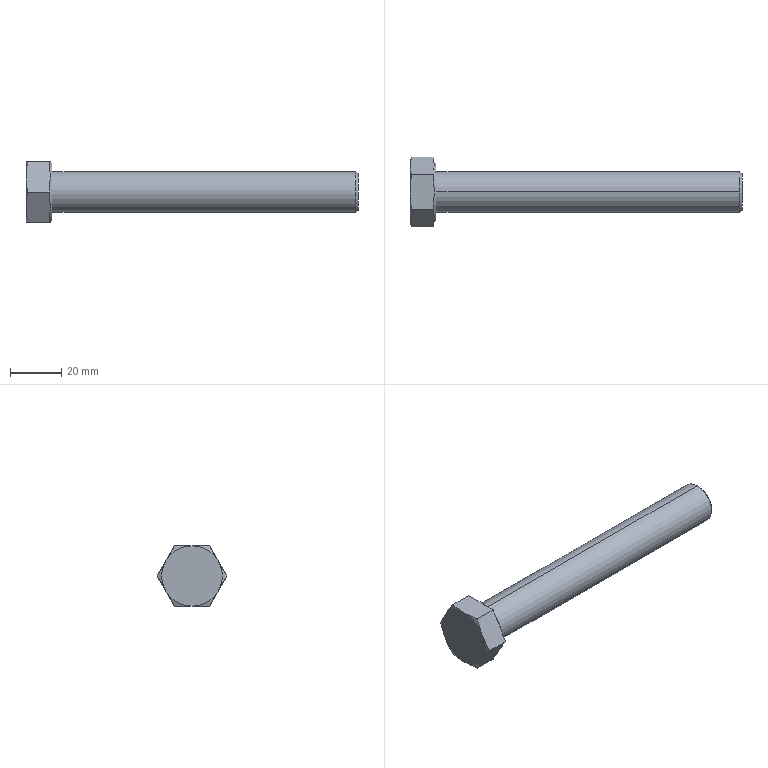Part | STEP file | hexagon head bolts-full thread_gb_GB_FASTENER_BOLT_STBAB A M16X120-N | 1 solid | 27 faces | box 130.18 x 27.332 x 23.67 mm | volume 28995 mm3 | plane 15 | cone 10 | cylinder 2 | commonest cylinder face diameters 16 x2